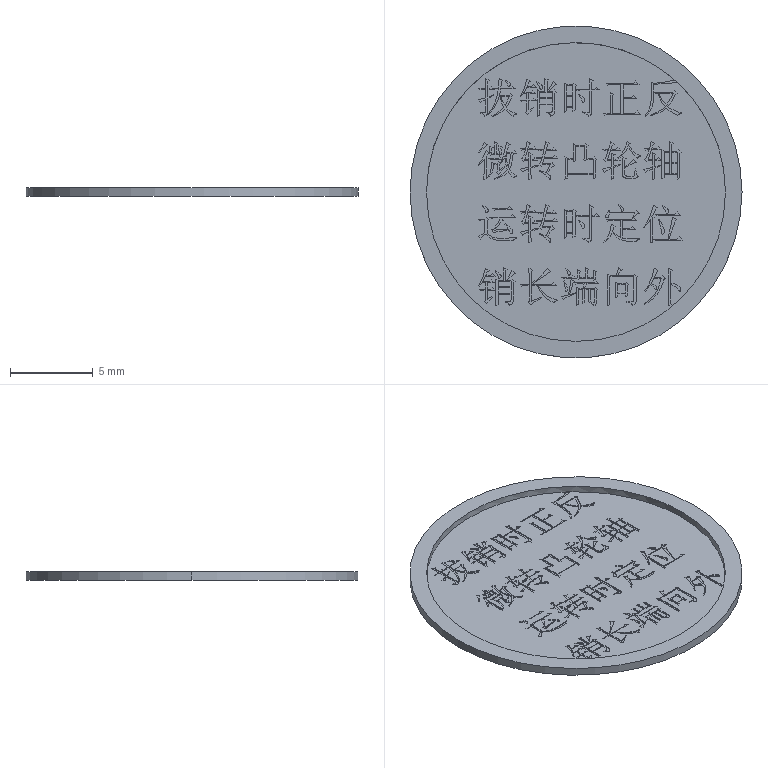Part | SolidWorks | features BaseBody 1 | 1 solid | 1070 faces | box 20 x 20 x 0.5 mm | volume 54.266 mm3 | plane 809 | spline 257 | cylinder 4 | commonest cylinder face diameters 18 x2 20 x2